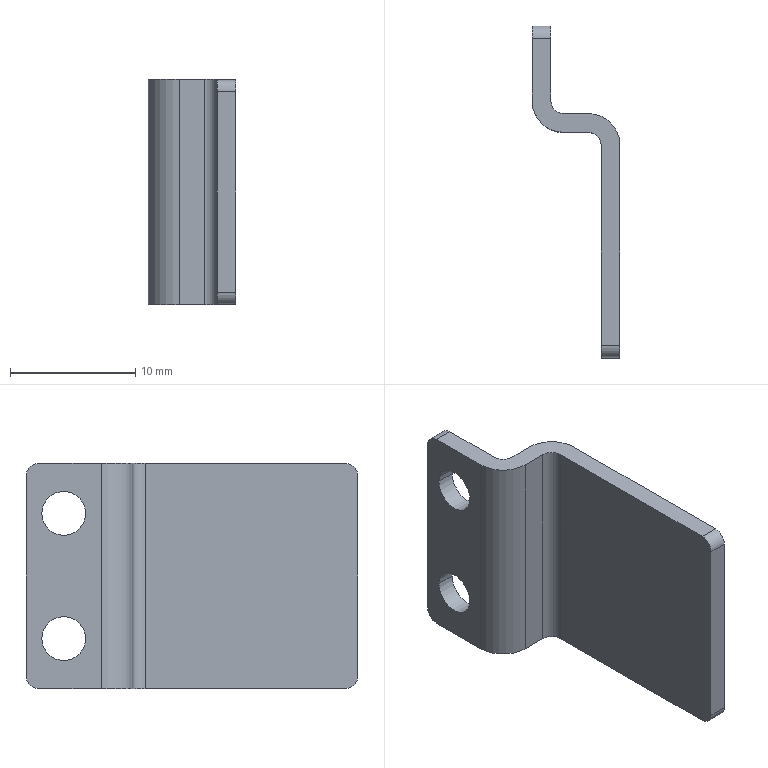Part | SolidWorks | features BaseBody 1 | 1 solid | 22 faces | box 7 x 26.5 x 18 mm | volume 793.289 mm3 | cylinder 12 | plane 10 | commonest cylinder face diameters 2 x6 3.5 x4 5 x2
STEP:
#1=CARTESIAN_POINT('',(-1.5,-4.75,5.));
#2=VERTEX_POINT('',#1);
#3=CARTESIAN_POINT('',(-1.5,-1.25,5.));
#4=VERTEX_POINT('',#3);
#5=CARTESIAN_POINT('',(-1.5,-3.,5.));
#6=DIRECTION('',(1.,0.,0.));
#7=DIRECTION('',(0.,1.,0.));
#8=AXIS2_PLACEMENT_3D('',#5,#6,#7);
#9=CIRCLE('',#8,1.75);
#10=EDGE_CURVE('',#2,#4,#9,.T.);
#11=ORIENTED_EDGE('',*,*,#10,.F.);
#12=CARTESIAN_POINT('',(0.,-4.75,5.));
#13=VERTEX_POINT('',#12);
#14=CARTESIAN_POINT('',(-10.,-4.75,5.));
#15=DIRECTION('',(1.,0.,0.));
#16=VECTOR('',#15,1000.);
#17=LINE('',#14,#16);
#18=EDGE_CURVE('',#2,#13,#17,.T.);
#19=ORIENTED_EDGE('',*,*,#18,.T.);
#20=CARTESIAN_POINT('',(0.,-1.25,5.));
#21=VERTEX_POINT('',#20);
#22=CARTESIAN_POINT('',(0.,-3.,5.));
#23=DIRECTION('',(-1.,0.,0.));
#24=DIRECTION('',(0.,1.,0.));
#25=AXIS2_PLACEMENT_3D('',#22,#23,#24);
#26=CIRCLE('',#25,1.75);
#27=EDGE_CURVE('',#21,#13,#26,.T.);
#28=ORIENTED_EDGE('',*,*,#27,.F.);
#29=CARTESIAN_POINT('',(-10.,-1.25,5.));
#30=DIRECTION('',(1.,0.,0.));
#31=VECTOR('',#30,1000.);
#32=LINE('',#29,#31);
#33=EDGE_CURVE('',#4,#21,#32,.T.);
#34=ORIENTED_EDGE('',*,*,#33,.F.);
#35=EDGE_LOOP('',(#11,#19,#28,#34));
#36=FACE_OUTER_BOUND('',#35,.T.);
#37=CARTESIAN_POINT('',(-10.,-3.,5.));
#38=DIRECTION('',(1.,0.,0.));
#39=DIRECTION('',(0.,1.,0.));
#40=AXIS2_PLACEMENT_3D('',#37,#38,#39);
#41=CYLINDRICAL_SURFACE('',#40,1.75);
#42=ADVANCED_FACE('',(#36),#41,.F.);
#43=CARTESIAN_POINT('',(-1.5,-4.75,-5.));
#44=VERTEX_POINT('',#43);
#45=CARTESIAN_POINT('',(-1.5,-1.25,-5.));
#46=VERTEX_POINT('',#45);
#47=CARTESIAN_POINT('',(-1.5,-3.,-5.));
#48=DIRECTION('',(1.,0.,0.));
#49=DIRECTION('',(0.,1.,0.));
#50=AXIS2_PLACEMENT_3D('',#47,#48,#49);
#51=CIRCLE('',#50,1.75);
#52=EDGE_CURVE('',#44,#46,#51,.T.);
#53=ORIENTED_EDGE('',*,*,#52,.F.);
#54=CARTESIAN_POINT('',(0.,-4.75,-5.));
#55=VERTEX_POINT('',#54);
#56=CARTESIAN_POINT('',(-10.,-4.75,-5.));
#57=DIRECTION('',(1.,0.,0.));
#58=VECTOR('',#57,1000.);
#59=LINE('',#56,#58);
#60=EDGE_CURVE('',#44,#55,#59,.T.);
#61=ORIENTED_EDGE('',*,*,#60,.T.);
#62=CARTESIAN_POINT('',(0.,-1.25,-5.));
#63=VERTEX_POINT('',#62);
#64=CARTESIAN_POINT('',(0.,-3.,-5.));
#65=DIRECTION('',(-1.,0.,0.));
#66=DIRECTION('',(0.,1.,0.));
#67=AXIS2_PLACEMENT_3D('',#64,#65,#66);
#68=CIRCLE('',#67,1.75);
#69=EDGE_CURVE('',#63,#55,#68,.T.);
#70=ORIENTED_EDGE('',*,*,#69,.F.);
#71=CARTESIAN_POINT('',(-10.,-1.25,-5.));
#72=DIRECTION('',(1.,0.,0.));
#73=VECTOR('',#72,1000.);
#74=LINE('',#71,#73);
#75=EDGE_CURVE('',#46,#63,#74,.T.);
#76=ORIENTED_EDGE('',*,*,#75,.F.);
#77=EDGE_LOOP('',(#53,#61,#70,#76));
#78=FACE_OUTER_BOUND('',#77,.T.);
#79=CARTESIAN_POINT('',(-10.,-3.,-5.));
#80=DIRECTION('',(1.,0.,0.));
#81=DIRECTION('',(0.,1.,0.));
#82=AXIS2_PLACEMENT_3D('',#79,#80,#81);
#83=CYLINDRICAL_SURFACE('',#82,1.75);
#84=ADVANCED_FACE('',(#78),#83,.F.);
#85=CARTESIAN_POINT('',(5.5,-25.5,-9.));
#86=VERTEX_POINT('',#85);
#87=CARTESIAN_POINT('',(5.5,-9.5,-9.));
#88=VERTEX_POINT('',#87);
#89=CARTESIAN_POINT('',(5.5,-7.,-9.));
#90=DIRECTION('',(0.,1.,0.));
#91=VECTOR('',#90,1000.);
#92=LINE('',#89,#91);
#93=EDGE_CURVE('',#86,#88,#92,.T.);
#94=ORIENTED_EDGE('',*,*,#93,.T.);
#95=CARTESIAN_POINT('',(5.5,-9.5,9.));
#96=VERTEX_POINT('',#95);
#97=CARTESIAN_POINT('',(5.5,-9.5,9.));
#98=DIRECTION('',(0.,0.,1.));
#99=VECTOR('',#98,1000.);
#100=LINE('',#97,#99);
#101=EDGE_CURVE('',#88,#96,#100,.T.);
#102=ORIENTED_EDGE('',*,*,#101,.T.);
#103=CARTESIAN_POINT('',(5.5,-25.5,9.));
#104=VERTEX_POINT('',#103);
#105=CARTESIAN_POINT('',(5.5,-7.,9.));
#106=DIRECTION('',(0.,-1.,0.));
#107=VECTOR('',#106,1000.);
#108=LINE('',#105,#107);
#109=EDGE_CURVE('',#96,#104,#108,.T.);
#110=ORIENTED_EDGE('',*,*,#109,.T.);
#111=CARTESIAN_POINT('',(5.5,-26.5,8.));
#112=VERTEX_POINT('',#111);
#113=CARTESIAN_POINT('',(5.5,-25.5,8.));
#114=DIRECTION('',(1.,0.,0.));
#115=DIRECTION('',(0.,0.,1.));
#116=AXIS2_PLACEMENT_3D('',#113,#114,#115);
#117=CIRCLE('',#116,1.);
#118=EDGE_CURVE('',#104,#112,#117,.T.);
#119=ORIENTED_EDGE('',*,*,#118,.T.);
#120=CARTESIAN_POINT('',(5.5,-26.5,-8.));
#121=VERTEX_POINT('',#120);
#122=CARTESIAN_POINT('',(5.5,-26.5,9.));
#123=DIRECTION('',(0.,0.,-1.));
#124=VECTOR('',#123,1000.);
#125=LINE('',#122,#124);
#126=EDGE_CURVE('',#112,#121,#125,.T.);
#127=ORIENTED_EDGE('',*,*,#126,.T.);
#128=CARTESIAN_POINT('',(5.5,-25.5,-8.));
#129=DIRECTION('',(1.,0.,0.));
#130=DIRECTION('',(0.,0.,-1.));
#131=AXIS2_PLACEMENT_3D('',#128,#129,#130);
#132=CIRCLE('',#131,1.);
#133=EDGE_CURVE('',#121,#86,#132,.T.);
#134=ORIENTED_EDGE('',*,*,#133,.T.);
#135=EDGE_LOOP('',(#94,#102,#110,#119,#127,#134));
#136=FACE_OUTER_BOUND('',#135,.T.);
#137=CARTESIAN_POINT('',(5.5,-7.,9.));
#138=DIRECTION('',(1.,0.,0.));
#139=DIRECTION('',(0.,1.,0.));
#140=AXIS2_PLACEMENT_3D('',#137,#138,#139);
#141=PLANE('',#140);
#142=ADVANCED_FACE('',(#136),#141,.T.);
#143=CARTESIAN_POINT('',(3.,-7.,9.));
#144=VERTEX_POINT('',#143);
#145=CARTESIAN_POINT('',(3.,-9.5,9.));
#146=DIRECTION('',(0.,0.,-1.));
#147=DIRECTION('',(-1.,0.,0.));
#148=AXIS2_PLACEMENT_3D('',#145,#146,#147);
#149=CIRCLE('',#148,2.5);
#150=EDGE_CURVE('',#144,#96,#149,.T.);
#151=ORIENTED_EDGE('',*,*,#150,.T.);
#152=ORIENTED_EDGE('',*,*,#101,.F.);
#153=CARTESIAN_POINT('',(3.,-7.,-9.));
#154=VERTEX_POINT('',#153);
#155=CARTESIAN_POINT('',(3.,-9.5,-9.));
#156=DIRECTION('',(0.,0.,1.));
#157=DIRECTION('',(-1.,0.,0.));
#158=AXIS2_PLACEMENT_3D('',#155,#156,#157);
#159=CIRCLE('',#158,2.5);
#160=EDGE_CURVE('',#88,#154,#159,.T.);
#161=ORIENTED_EDGE('',*,*,#160,.T.);
#162=CARTESIAN_POINT('',(3.,-7.,9.));
#163=DIRECTION('',(0.,0.,1.));
#164=VECTOR('',#163,1000.);
#165=LINE('',#162,#164);
#166=EDGE_CURVE('',#154,#144,#165,.T.);
#167=ORIENTED_EDGE('',*,*,#166,.T.);
#168=EDGE_LOOP('',(#151,#152,#161,#167));
#169=FACE_OUTER_BOUND('',#168,.T.);
#170=CARTESIAN_POINT('',(3.,-9.5,9.));
#171=DIRECTION('',(0.,0.,-1.));
#172=DIRECTION('',(-1.,0.,0.));
#173=AXIS2_PLACEMENT_3D('',#170,#171,#172);
#174=CYLINDRICAL_SURFACE('',#173,2.5);
#175=ADVANCED_FACE('',(#169),#174,.T.);
#176=CARTESIAN_POINT('',(4.,-25.5,-9.));
#177=VERTEX_POINT('',#176);
#178=CARTESIAN_POINT('',(3.,-25.5,-9.));
#179=DIRECTION('',(1.,0.,0.));
#180=VECTOR('',#179,1000.);
#181=LINE('',#178,#180);
#182=EDGE_CURVE('',#177,#86,#181,.T.);
#183=ORIENTED_EDGE('',*,*,#182,.F.);
#184=CARTESIAN_POINT('',(4.,-9.5,-9.));
#185=VERTEX_POINT('',#184);
#186=CARTESIAN_POINT('',(4.,-9.5,-9.));
#187=DIRECTION('',(0.,-1.,0.));
#188=VECTOR('',#187,1000.);
#189=LINE('',#186,#188);
#190=EDGE_CURVE('',#185,#177,#189,.T.);
#191=ORIENTED_EDGE('',*,*,#190,.F.);
#192=CARTESIAN_POINT('',(3.,-8.5,-9.));
#193=VERTEX_POINT('',#192);
#194=CARTESIAN_POINT('',(3.,-9.5,-9.));
#195=DIRECTION('',(0.,0.,1.));
#196=DIRECTION('',(-1.,0.,0.));
#197=AXIS2_PLACEMENT_3D('',#194,#195,#196);
#198=CIRCLE('',#197,1.);
#199=EDGE_CURVE('',#185,#193,#198,.T.);
#200=ORIENTED_EDGE('',*,*,#199,.T.);
#201=CARTESIAN_POINT('',(1.,-8.5,-9.));
#202=VERTEX_POINT('',#201);
#203=CARTESIAN_POINT('',(4.,-8.5,-9.));
#204=DIRECTION('',(-1.,0.,0.));
#205=VECTOR('',#204,1000.);
#206=LINE('',#203,#205);
#207=EDGE_CURVE('',#193,#202,#206,.T.);
#208=ORIENTED_EDGE('',*,*,#207,.T.);
#209=CARTESIAN_POINT('',(-1.5,-6.,-9.));
#210=VERTEX_POINT('',#209);
#211=CARTESIAN_POINT('',(1.,-6.,-9.));
#212=DIRECTION('',(0.,0.,1.));
#213=DIRECTION('',(-1.,0.,0.));
#214=AXIS2_PLACEMENT_3D('',#211,#212,#213);
#215=CIRCLE('',#214,2.5);
#216=EDGE_CURVE('',#210,#202,#215,.T.);
#217=ORIENTED_EDGE('',*,*,#216,.F.);
#218=CARTESIAN_POINT('',(-1.5,-1.,-9.));
#219=VERTEX_POINT('',#218);
#220=CARTESIAN_POINT('',(-1.5,-8.5,-9.));
#221=DIRECTION('',(0.,1.,0.));
#222=VECTOR('',#221,1000.);
#223=LINE('',#220,#222);
#224=EDGE_CURVE('',#210,#219,#223,.T.);
#225=ORIENTED_EDGE('',*,*,#224,.T.);
#226=CARTESIAN_POINT('',(0.,-1.,-9.));
#227=VERTEX_POINT('',#226);
#228=CARTESIAN_POINT('',(1.,-1.,-9.));
#229=DIRECTION('',(-1.,0.,0.));
#230=VECTOR('',#229,1000.);
#231=LINE('',#228,#230);
#232=EDGE_CURVE('',#227,#219,#231,.T.);
#233=ORIENTED_EDGE('',*,*,#232,.F.);
#234=CARTESIAN_POINT('',(0.,-6.,-9.));
#235=VERTEX_POINT('',#234);
#236=CARTESIAN_POINT('',(0.,0.,-9.));
#237=DIRECTION('',(0.,1.,0.));
#238=VECTOR('',#237,1000.);
#239=LINE('',#236,#238);
#240=EDGE_CURVE('',#235,#227,#239,.T.);
#241=ORIENTED_EDGE('',*,*,#240,.F.);
#242=CARTESIAN_POINT('',(1.,-7.,-9.));
#243=VERTEX_POINT('',#242);
#244=CARTESIAN_POINT('',(1.,-6.,-9.));
#245=DIRECTION('',(0.,0.,1.));
#246=DIRECTION('',(-1.,0.,0.));
#247=AXIS2_PLACEMENT_3D('',#244,#245,#246);
#248=CIRCLE('',#247,1.);
#249=EDGE_CURVE('',#235,#243,#248,.T.);
#250=ORIENTED_EDGE('',*,*,#249,.T.);
#251=CARTESIAN_POINT('',(0.,-7.,-9.));
#252=DIRECTION('',(-1.,0.,0.));
#253=VECTOR('',#252,1000.);
#254=LINE('',#251,#253);
#255=EDGE_CURVE('',#154,#243,#254,.T.);
#256=ORIENTED_EDGE('',*,*,#255,.F.);
#257=ORIENTED_EDGE('',*,*,#160,.F.);
#258=ORIENTED_EDGE('',*,*,#93,.F.);
#259=EDGE_LOOP('',(#183,#191,#200,#208,#217,#225,#233,#241,#250,#256,#257,#258));
#260=FACE_OUTER_BOUND('',#259,.T.);
#261=CARTESIAN_POINT('',(3.,-9.5,-9.));
#262=DIRECTION('',(0.,0.,1.));
#263=DIRECTION('',(1.,0.,0.));
#264=AXIS2_PLACEMENT_3D('',#261,#262,#263);
#265=PLANE('',#264);
#266=ADVANCED_FACE('',(#260),#265,.F.);
#267=CARTESIAN_POINT('',(4.,-26.5,-8.));
#268=VERTEX_POINT('',#267);
#269=CARTESIAN_POINT('',(4.,-25.5,-8.));
#270=DIRECTION('',(1.,0.,0.));
#271=DIRECTION('',(0.,0.,-1.));
#272=AXIS2_PLACEMENT_3D('',#269,#270,#271);
#273=CIRCLE('',#272,1.);
#274=EDGE_CURVE('',#268,#177,#273,.T.);
#275=ORIENTED_EDGE('',*,*,#274,.T.);
#276=ORIENTED_EDGE('',*,*,#182,.T.);
#277=ORIENTED_EDGE('',*,*,#133,.F.);
#278=CARTESIAN_POINT('',(3.,-26.5,-8.));
#279=DIRECTION('',(-1.,0.,0.));
#280=VECTOR('',#279,1000.);
#281=LINE('',#278,#280);
#282=EDGE_CURVE('',#121,#268,#281,.T.);
#283=ORIENTED_EDGE('',*,*,#282,.T.);
#284=EDGE_LOOP('',(#275,#276,#277,#283));
#285=FACE_OUTER_BOUND('',#284,.T.);
#286=CARTESIAN_POINT('',(3.,-25.5,-8.));
#287=DIRECTION('',(1.,0.,0.));
#288=DIRECTION('',(0.,0.,-1.));
#289=AXIS2_PLACEMENT_3D('',#286,#287,#288);
#290=CYLINDRICAL_SURFACE('',#289,1.);
#291=ADVANCED_FACE('',(#285),#290,.T.);
#292=CARTESIAN_POINT('',(4.,-26.5,8.));
#293=VERTEX_POINT('',#292);
#294=CARTESIAN_POINT('',(4.,-26.5,9.));
#295=DIRECTION('',(0.,0.,-1.));
#296=VECTOR('',#295,1000.);
#297=LINE('',#294,#296);
#298=EDGE_CURVE('',#293,#268,#297,.T.);
#299=ORIENTED_EDGE('',*,*,#298,.T.);
#300=ORIENTED_EDGE('',*,*,#282,.F.);
#301=ORIENTED_EDGE('',*,*,#126,.F.);
#302=CARTESIAN_POINT('',(5.5,-26.5,8.));
#303=DIRECTION('',(-1.,0.,0.));
#304=VECTOR('',#303,1000.);
#305=LINE('',#302,#304);
#306=EDGE_CURVE('',#112,#293,#305,.T.);
#307=ORIENTED_EDGE('',*,*,#306,.T.);
#308=EDGE_LOOP('',(#299,#300,#301,#307));
#309=FACE_OUTER_BOUND('',#308,.T.);
#310=CARTESIAN_POINT('',(5.5,-26.5,9.));
#311=DIRECTION('',(0.,-1.,0.));
#312=DIRECTION('',(0.,0.,-1.));
#313=AXIS2_PLACEMENT_3D('',#310,#311,#312);
#314=PLANE('',#313);
#315=ADVANCED_FACE('',(#309),#314,.T.);
#316=CARTESIAN_POINT('',(4.,-25.5,9.));
#317=VERTEX_POINT('',#316);
#318=CARTESIAN_POINT('',(4.,-25.5,8.));
#319=DIRECTION('',(1.,0.,0.));
#320=DIRECTION('',(0.,0.,1.));
#321=AXIS2_PLACEMENT_3D('',#318,#319,#320);
#322=CIRCLE('',#321,1.);
#323=EDGE_CURVE('',#317,#293,#322,.T.);
#324=ORIENTED_EDGE('',*,*,#323,.T.);
#325=ORIENTED_EDGE('',*,*,#306,.F.);
#326=ORIENTED_EDGE('',*,*,#118,.F.);
#327=CARTESIAN_POINT('',(5.5,-25.5,9.));
#328=DIRECTION('',(-1.,0.,0.));
#329=VECTOR('',#328,1000.);
#330=LINE('',#327,#329);
#331=EDGE_CURVE('',#104,#317,#330,.T.);
#332=ORIENTED_EDGE('',*,*,#331,.T.);
#333=EDGE_LOOP('',(#324,#325,#326,#332));
#334=FACE_OUTER_BOUND('',#333,.T.);
#335=CARTESIAN_POINT('',(5.5,-25.5,8.));
#336=DIRECTION('',(-1.,0.,0.));
#337=DIRECTION('',(0.,0.,1.));
#338=AXIS2_PLACEMENT_3D('',#335,#336,#337);
#339=CYLINDRICAL_SURFACE('',#338,1.);
#340=ADVANCED_FACE('',(#334),#339,.T.);
#341=ORIENTED_EDGE('',*,*,#109,.F.);
#342=ORIENTED_EDGE('',*,*,#150,.F.);
#343=CARTESIAN_POINT('',(1.,-7.,9.));
#344=VERTEX_POINT('',#343);
#345=CARTESIAN_POINT('',(0.,-7.,9.));
#346=DIRECTION('',(1.,0.,0.));
#347=VECTOR('',#346,1000.);
#348=LINE('',#345,#347);
#349=EDGE_CURVE('',#344,#144,#348,.T.);
#350=ORIENTED_EDGE('',*,*,#349,.F.);
#351=CARTESIAN_POINT('',(0.,-6.,9.));
#352=VERTEX_POINT('',#351);
#353=CARTESIAN_POINT('',(1.,-6.,9.));
#354=DIRECTION('',(0.,0.,-1.));
#355=DIRECTION('',(-1.,0.,0.));
#356=AXIS2_PLACEMENT_3D('',#353,#354,#355);
#357=CIRCLE('',#356,1.);
#358=EDGE_CURVE('',#344,#352,#357,.T.);
#359=ORIENTED_EDGE('',*,*,#358,.T.);
#360=CARTESIAN_POINT('',(0.,-1.,9.));
#361=VERTEX_POINT('',#360);
#362=CARTESIAN_POINT('',(0.,0.,9.));
#363=DIRECTION('',(0.,-1.,0.));
#364=VECTOR('',#363,1000.);
#365=LINE('',#362,#364);
#366=EDGE_CURVE('',#361,#352,#365,.T.);
#367=ORIENTED_EDGE('',*,*,#366,.F.);
#368=CARTESIAN_POINT('',(-1.5,-1.,9.));
#369=VERTEX_POINT('',#368);
#370=CARTESIAN_POINT('',(3.,-1.,9.));
#371=DIRECTION('',(-1.,0.,0.));
#372=VECTOR('',#371,1000.);
#373=LINE('',#370,#372);
#374=EDGE_CURVE('',#361,#369,#373,.T.);
#375=ORIENTED_EDGE('',*,*,#374,.T.);
#376=CARTESIAN_POINT('',(-1.5,-6.,9.));
#377=VERTEX_POINT('',#376);
#378=CARTESIAN_POINT('',(-1.5,-9.5,9.));
#379=DIRECTION('',(0.,-1.,0.));
#380=VECTOR('',#379,1000.);
#381=LINE('',#378,#380);
#382=EDGE_CURVE('',#369,#377,#381,.T.);
#383=ORIENTED_EDGE('',*,*,#382,.T.);
#384=CARTESIAN_POINT('',(1.,-8.5,9.));
#385=VERTEX_POINT('',#384);
#386=CARTESIAN_POINT('',(1.,-6.,9.));
#387=DIRECTION('',(0.,0.,-1.));
#388=DIRECTION('',(-1.,0.,0.));
#389=AXIS2_PLACEMENT_3D('',#386,#387,#388);
#390=CIRCLE('',#389,2.5);
#391=EDGE_CURVE('',#385,#377,#390,.T.);
#392=ORIENTED_EDGE('',*,*,#391,.F.);
#393=CARTESIAN_POINT('',(3.,-8.5,9.));
#394=VERTEX_POINT('',#393);
#395=CARTESIAN_POINT('',(-1.5,-8.5,9.));
#396=DIRECTION('',(1.,0.,0.));
#397=VECTOR('',#396,1000.);
#398=LINE('',#395,#397);
#399=EDGE_CURVE('',#385,#394,#398,.T.);
#400=ORIENTED_EDGE('',*,*,#399,.T.);
#401=CARTESIAN_POINT('',(4.,-9.5,9.));
#402=VERTEX_POINT('',#401);
#403=CARTESIAN_POINT('',(3.,-9.5,9.));
#404=DIRECTION('',(0.,0.,-1.));
#405=DIRECTION('',(-1.,0.,0.));
#406=AXIS2_PLACEMENT_3D('',#403,#404,#405);
#407=CIRCLE('',#406,1.);
#408=EDGE_CURVE('',#394,#402,#407,.T.);
#409=ORIENTED_EDGE('',*,*,#408,.T.);
#410=CARTESIAN_POINT('',(4.,-8.5,9.));
#411=DIRECTION('',(0.,-1.,0.));
#412=VECTOR('',#411,1000.);
#413=LINE('',#410,#412);
#414=EDGE_CURVE('',#402,#317,#413,.T.);
#415=ORIENTED_EDGE('',*,*,#414,.T.);
#416=ORIENTED_EDGE('',*,*,#331,.F.);
#417=EDGE_LOOP('',(#341,#342,#350,#359,#367,#375,#383,#392,#400,#409,#415,#416));
#418=FACE_OUTER_BOUND('',#417,.T.);
#419=CARTESIAN_POINT('',(3.,-8.5,9.));
#420=DIRECTION('',(0.,0.,1.));
#421=DIRECTION('',(1.,0.,0.));
#422=AXIS2_PLACEMENT_3D('',#419,#420,#421);
#423=PLANE('',#422);
#424=ADVANCED_FACE('',(#418),#423,.T.);
#425=ORIENTED_EDGE('',*,*,#349,.T.);
#426=ORIENTED_EDGE('',*,*,#166,.F.);
#427=ORIENTED_EDGE('',*,*,#255,.T.);
#428=CARTESIAN_POINT('',(1.,-7.,9.));
#429=DIRECTION('',(0.,0.,1.));
#430=VECTOR('',#429,1000.);
#431=LINE('',#428,#430);
#432=EDGE_CURVE('',#243,#344,#431,.T.);
#433=ORIENTED_EDGE('',*,*,#432,.T.);
#434=EDGE_LOOP('',(#425,#426,#427,#433));
#435=FACE_OUTER_BOUND('',#434,.T.);
#436=CARTESIAN_POINT('',(0.,-7.,9.));
#437=DIRECTION('',(0.,1.,0.));
#438=DIRECTION('',(0.,0.,1.));
#439=AXIS2_PLACEMENT_3D('',#436,#437,#438);
#440=PLANE('',#439);
#441=ADVANCED_FACE('',(#435),#440,.T.);
#442=ORIENTED_EDGE('',*,*,#323,.F.);
#443=ORIENTED_EDGE('',*,*,#414,.F.);
#444=CARTESIAN_POINT('',(4.,-9.5,9.));
#445=DIRECTION('',(0.,0.,1.));
#446=VECTOR('',#445,1000.);
#447=LINE('',#444,#446);
#448=EDGE_CURVE('',#185,#402,#447,.T.);
#449=ORIENTED_EDGE('',*,*,#448,.F.);
#450=ORIENTED_EDGE('',*,*,#190,.T.);
#451=ORIENTED_EDGE('',*,*,#274,.F.);
#452=ORIENTED_EDGE('',*,*,#298,.F.);
#453=EDGE_LOOP('',(#442,#443,#449,#450,#451,#452));
#454=FACE_OUTER_BOUND('',#453,.T.);
#455=CARTESIAN_POINT('',(4.,-7.,9.));
#456=DIRECTION('',(1.,0.,0.));
#457=DIRECTION('',(0.,1.,0.));
#458=AXIS2_PLACEMENT_3D('',#455,#456,#457);
#459=PLANE('',#458);
#460=ADVANCED_FACE('',(#454),#459,.F.);
#461=CARTESIAN_POINT('',(0.,-6.,9.));
#462=DIRECTION('',(0.,0.,-1.));
#463=VECTOR('',#462,1000.);
#464=LINE('',#461,#463);
#465=EDGE_CURVE('',#352,#235,#464,.T.);
#466=ORIENTED_EDGE('',*,*,#465,.F.);
#467=ORIENTED_EDGE('',*,*,#358,.F.);
#468=ORIENTED_EDGE('',*,*,#432,.F.);
#469=ORIENTED_EDGE('',*,*,#249,.F.);
#470=EDGE_LOOP('',(#466,#467,#468,#469));
#471=FACE_OUTER_BOUND('',#470,.T.);
#472=CARTESIAN_POINT('',(1.,-6.,9.));
#473=DIRECTION('',(0.,0.,-1.));
#474=DIRECTION('',(-1.,0.,0.));
#475=AXIS2_PLACEMENT_3D('',#472,#473,#474);
#476=CYLINDRICAL_SURFACE('',#475,1.);
#477=ADVANCED_FACE('',(#471),#476,.F.);
#478=ORIENTED_EDGE('',*,*,#448,.T.);
#479=ORIENTED_EDGE('',*,*,#408,.F.);
#480=CARTESIAN_POINT('',(3.,-8.5,9.));
#481=DIRECTION('',(0.,0.,1.));
#482=VECTOR('',#481,1000.);
#483=LINE('',#480,#482);
#484=EDGE_CURVE('',#193,#394,#483,.T.);
#485=ORIENTED_EDGE('',*,*,#484,.F.);
#486=ORIENTED_EDGE('',*,*,#199,.F.);
#487=EDGE_LOOP('',(#478,#479,#485,#486));
#488=FACE_OUTER_BOUND('',#487,.T.);
#489=CARTESIAN_POINT('',(3.,-9.5,9.));
#490=DIRECTION('',(0.,0.,-1.));
#491=DIRECTION('',(-1.,0.,0.));
#492=AXIS2_PLACEMENT_3D('',#489,#490,#491);
#493=CYLINDRICAL_SURFACE('',#492,1.);
#494=ADVANCED_FACE('',(#488),#493,.F.);
#495=ORIENTED_EDGE('',*,*,#484,.T.);
#496=ORIENTED_EDGE('',*,*,#399,.F.);
#497=CARTESIAN_POINT('',(1.,-8.5,9.));
#498=DIRECTION('',(0.,0.,1.));
#499=VECTOR('',#498,1000.);
#500=LINE('',#497,#499);
#501=EDGE_CURVE('',#202,#385,#500,.T.);
#502=ORIENTED_EDGE('',*,*,#501,.F.);
#503=ORIENTED_EDGE('',*,*,#207,.F.);
#504=EDGE_LOOP('',(#495,#496,#502,#503));
#505=FACE_OUTER_BOUND('',#504,.T.);
#506=CARTESIAN_POINT('',(0.,-8.5,9.));
#507=DIRECTION('',(0.,1.,0.));
#508=DIRECTION('',(0.,0.,1.));
#509=AXIS2_PLACEMENT_3D('',#506,#507,#508);
#510=PLANE('',#509);
#511=ADVANCED_FACE('',(#505),#510,.F.);
#512=ORIENTED_EDGE('',*,*,#366,.T.);
#513=ORIENTED_EDGE('',*,*,#465,.T.);
#514=ORIENTED_EDGE('',*,*,#240,.T.);
#515=CARTESIAN_POINT('',(0.,0.,-8.));
#516=VERTEX_POINT('',#515);
#517=CARTESIAN_POINT('',(0.,-1.,-8.));
#518=DIRECTION('',(1.,0.,0.));
#519=DIRECTION('',(0.,1.,0.));
#520=AXIS2_PLACEMENT_3D('',#517,#518,#519);
#521=CIRCLE('',#520,1.);
#522=EDGE_CURVE('',#227,#516,#521,.T.);
#523=ORIENTED_EDGE('',*,*,#522,.T.);
#524=CARTESIAN_POINT('',(0.,0.,8.));
#525=VERTEX_POINT('',#524);
#526=CARTESIAN_POINT('',(0.,0.,9.));
#527=DIRECTION('',(0.,0.,1.));
#528=VECTOR('',#527,1000.);
#529=LINE('',#526,#528);
#530=EDGE_CURVE('',#516,#525,#529,.T.);
#531=ORIENTED_EDGE('',*,*,#530,.T.);
#532=CARTESIAN_POINT('',(0.,-1.,8.));
#533=DIRECTION('',(1.,0.,0.));
#534=DIRECTION('',(0.,1.,0.));
#535=AXIS2_PLACEMENT_3D('',#532,#533,#534);
#536=CIRCLE('',#535,1.);
#537=EDGE_CURVE('',#525,#361,#536,.T.);
#538=ORIENTED_EDGE('',*,*,#537,.T.);
#539=EDGE_LOOP('',(#512,#513,#514,#523,#531,#538));
#540=FACE_OUTER_BOUND('',#539,.T.);
#541=ORIENTED_EDGE('',*,*,#27,.T.);
#542=CARTESIAN_POINT('',(0.,-3.,5.));
#543=DIRECTION('',(-1.,0.,0.));
#544=DIRECTION('',(0.,1.,0.));
#545=AXIS2_PLACEMENT_3D('',#542,#543,#544);
#546=CIRCLE('',#545,1.75);
#547=EDGE_CURVE('',#13,#21,#546,.T.);
#548=ORIENTED_EDGE('',*,*,#547,.T.);
#549=EDGE_LOOP('',(#541,#548));
#550=FACE_BOUND('',#549,.T.);
#551=ORIENTED_EDGE('',*,*,#69,.T.);
#552=CARTESIAN_POINT('',(0.,-3.,-5.));
#553=DIRECTION('',(-1.,0.,0.));
#554=DIRECTION('',(0.,1.,0.));
#555=AXIS2_PLACEMENT_3D('',#552,#553,#554);
#556=CIRCLE('',#555,1.75);
#557=EDGE_CURVE('',#55,#63,#556,.T.);
#558=ORIENTED_EDGE('',*,*,#557,.T.);
#559=EDGE_LOOP('',(#551,#558));
#560=FACE_BOUND('',#559,.T.);
#561=CARTESIAN_POINT('',(0.,0.,9.));
#562=DIRECTION('',(1.,0.,0.));
#563=DIRECTION('',(0.,1.,0.));
#564=AXIS2_PLACEMENT_3D('',#561,#562,#563);
#565=PLANE('',#564);
#566=ADVANCED_FACE('',(#540,#550,#560),#565,.T.);
#567=ORIENTED_EDGE('',*,*,#391,.T.);
#568=CARTESIAN_POINT('',(-1.5,-6.,9.));
#569=DIRECTION('',(0.,0.,-1.));
#570=VECTOR('',#569,1000.);
#571=LINE('',#568,#570);
#572=EDGE_CURVE('',#377,#210,#571,.T.);
#573=ORIENTED_EDGE('',*,*,#572,.T.);
#574=ORIENTED_EDGE('',*,*,#216,.T.);
#575=ORIENTED_EDGE('',*,*,#501,.T.);
#576=EDGE_LOOP('',(#567,#573,#574,#575));
#577=FACE_OUTER_BOUND('',#576,.T.);
#578=CARTESIAN_POINT('',(1.,-6.,9.));
#579=DIRECTION('',(0.,0.,-1.));
#580=DIRECTION('',(-1.,0.,0.));
#581=AXIS2_PLACEMENT_3D('',#578,#579,#580);
#582=CYLINDRICAL_SURFACE('',#581,2.5);
#583=ADVANCED_FACE('',(#577),#582,.T.);
#584=ORIENTED_EDGE('',*,*,#537,.F.);
#585=CARTESIAN_POINT('',(-1.5,0.,8.));
#586=VERTEX_POINT('',#585);
#587=CARTESIAN_POINT('',(-1.5,0.,8.));
#588=DIRECTION('',(-1.,0.,0.));
#589=VECTOR('',#588,1000.);
#590=LINE('',#587,#589);
#591=EDGE_CURVE('',#525,#586,#590,.T.);
#592=ORIENTED_EDGE('',*,*,#591,.T.);
#593=CARTESIAN_POINT('',(-1.5,-1.,8.));
#594=DIRECTION('',(1.,0.,0.));
#595=DIRECTION('',(0.,1.,0.));
#596=AXIS2_PLACEMENT_3D('',#593,#594,#595);
#597=CIRCLE('',#596,1.);
#598=EDGE_CURVE('',#586,#369,#597,.T.);
#599=ORIENTED_EDGE('',*,*,#598,.T.);
#600=ORIENTED_EDGE('',*,*,#374,.F.);
#601=EDGE_LOOP('',(#584,#592,#599,#600));
#602=FACE_OUTER_BOUND('',#601,.T.);
#603=CARTESIAN_POINT('',(-1.5,-1.,8.));
#604=DIRECTION('',(1.,0.,0.));
#605=DIRECTION('',(0.,1.,0.));
#606=AXIS2_PLACEMENT_3D('',#603,#604,#605);
#607=CYLINDRICAL_SURFACE('',#606,1.);
#608=ADVANCED_FACE('',(#602),#607,.T.);
#609=CARTESIAN_POINT('',(-1.5,0.,-8.));
#610=VERTEX_POINT('',#609);
#611=CARTESIAN_POINT('',(-1.5,0.,9.));
#612=DIRECTION('',(0.,0.,1.));
#613=VECTOR('',#612,1000.);
#614=LINE('',#611,#613);
#615=EDGE_CURVE('',#610,#586,#614,.T.);
#616=ORIENTED_EDGE('',*,*,#615,.T.);
#617=ORIENTED_EDGE('',*,*,#591,.F.);
#618=ORIENTED_EDGE('',*,*,#530,.F.);
#619=CARTESIAN_POINT('',(-1.5,0.,-8.));
#620=DIRECTION('',(-1.,0.,0.));
#621=VECTOR('',#620,1000.);
#622=LINE('',#619,#621);
#623=EDGE_CURVE('',#516,#610,#622,.T.);
#624=ORIENTED_EDGE('',*,*,#623,.T.);
#625=EDGE_LOOP('',(#616,#617,#618,#624));
#626=FACE_OUTER_BOUND('',#625,.T.);
#627=CARTESIAN_POINT('',(-1.5,0.,9.));
#628=DIRECTION('',(0.,1.,0.));
#629=DIRECTION('',(-1.,0.,0.));
#630=AXIS2_PLACEMENT_3D('',#627,#628,#629);
#631=PLANE('',#630);
#632=ADVANCED_FACE('',(#626),#631,.T.);
#633=ORIENTED_EDGE('',*,*,#522,.F.);
#634=ORIENTED_EDGE('',*,*,#232,.T.);
#635=CARTESIAN_POINT('',(-1.5,-1.,-8.));
#636=DIRECTION('',(1.,0.,0.));
#637=DIRECTION('',(0.,1.,0.));
#638=AXIS2_PLACEMENT_3D('',#635,#636,#637);
#639=CIRCLE('',#638,1.);
#640=EDGE_CURVE('',#219,#610,#639,.T.);
#641=ORIENTED_EDGE('',*,*,#640,.T.);
#642=ORIENTED_EDGE('',*,*,#623,.F.);
#643=EDGE_LOOP('',(#633,#634,#641,#642));
#644=FACE_OUTER_BOUND('',#643,.T.);
#645=CARTESIAN_POINT('',(1.,-1.,-8.));
#646=DIRECTION('',(1.,0.,0.));
#647=DIRECTION('',(0.,1.,0.));
#648=AXIS2_PLACEMENT_3D('',#645,#646,#647);
#649=CYLINDRICAL_SURFACE('',#648,1.);
#650=ADVANCED_FACE('',(#644),#649,.T.);
#651=ORIENTED_EDGE('',*,*,#18,.F.);
#652=CARTESIAN_POINT('',(-1.5,-3.,5.));
#653=DIRECTION('',(1.,0.,0.));
#654=DIRECTION('',(0.,1.,0.));
#655=AXIS2_PLACEMENT_3D('',#652,#653,#654);
#656=CIRCLE('',#655,1.75);
#657=EDGE_CURVE('',#4,#2,#656,.T.);
#658=ORIENTED_EDGE('',*,*,#657,.F.);
#659=ORIENTED_EDGE('',*,*,#33,.T.);
#660=ORIENTED_EDGE('',*,*,#547,.F.);
#661=EDGE_LOOP('',(#651,#658,#659,#660));
#662=FACE_OUTER_BOUND('',#661,.T.);
#663=CARTESIAN_POINT('',(-10.,-3.,5.));
#664=DIRECTION('',(1.,0.,0.));
#665=DIRECTION('',(0.,1.,0.));
#666=AXIS2_PLACEMENT_3D('',#663,#664,#665);
#667=CYLINDRICAL_SURFACE('',#666,1.75);
#668=ADVANCED_FACE('',(#662),#667,.F.);
#669=ORIENTED_EDGE('',*,*,#60,.F.);
#670=CARTESIAN_POINT('',(-1.5,-3.,-5.));
#671=DIRECTION('',(1.,0.,0.));
#672=DIRECTION('',(0.,1.,0.));
#673=AXIS2_PLACEMENT_3D('',#670,#671,#672);
#674=CIRCLE('',#673,1.75);
#675=EDGE_CURVE('',#46,#44,#674,.T.);
#676=ORIENTED_EDGE('',*,*,#675,.F.);
#677=ORIENTED_EDGE('',*,*,#75,.T.);
#678=ORIENTED_EDGE('',*,*,#557,.F.);
#679=EDGE_LOOP('',(#669,#676,#677,#678));
#680=FACE_OUTER_BOUND('',#679,.T.);
#681=CARTESIAN_POINT('',(-10.,-3.,-5.));
#682=DIRECTION('',(1.,0.,0.));
#683=DIRECTION('',(0.,1.,0.));
#684=AXIS2_PLACEMENT_3D('',#681,#682,#683);
#685=CYLINDRICAL_SURFACE('',#684,1.75);
#686=ADVANCED_FACE('',(#680),#685,.F.);
#687=ORIENTED_EDGE('',*,*,#640,.F.);
#688=ORIENTED_EDGE('',*,*,#224,.F.);
#689=ORIENTED_EDGE('',*,*,#572,.F.);
#690=ORIENTED_EDGE('',*,*,#382,.F.);
#691=ORIENTED_EDGE('',*,*,#598,.F.);
#692=ORIENTED_EDGE('',*,*,#615,.F.);
#693=EDGE_LOOP('',(#687,#688,#689,#690,#691,#692));
#694=FACE_OUTER_BOUND('',#693,.T.);
#695=ORIENTED_EDGE('',*,*,#657,.T.);
#696=ORIENTED_EDGE('',*,*,#10,.T.);
#697=EDGE_LOOP('',(#695,#696));
#698=FACE_BOUND('',#697,.T.);
#699=ORIENTED_EDGE('',*,*,#675,.T.);
#700=ORIENTED_EDGE('',*,*,#52,.T.);
#701=EDGE_LOOP('',(#699,#700));
#702=FACE_BOUND('',#701,.T.);
#703=CARTESIAN_POINT('',(-1.5,0.,9.));
#704=DIRECTION('',(1.,0.,0.));
#705=DIRECTION('',(0.,1.,0.));
#706=AXIS2_PLACEMENT_3D('',#703,#704,#705);
#707=PLANE('',#706);
#708=ADVANCED_FACE('',(#694,#698,#702),#707,.F.);
#709=CLOSED_SHELL('',(#42,#84,#142,#175,#266,#291,#315,#340,#424,#441,#460,#477,#494,#511,#566,#583,#608,#632,#650,#668,#686,#708));
#710=MANIFOLD_SOLID_BREP('',#709);
#711=CARTESIAN_POINT('',(0.,0.,0.));
#712=DIRECTION('',(0.,0.,1.));
#713=DIRECTION('',(1.,0.,0.));
#714=AXIS2_PLACEMENT_3D('',#711,#712,#713);
#715=(LENGTH_UNIT()NAMED_UNIT(*)SI_UNIT(.MILLI.,.METRE.));
#716=UNCERTAINTY_MEASURE_WITH_UNIT(LENGTH_MEASURE(0.00001),#715,'','');
#717=(NAMED_UNIT(*)PLANE_ANGLE_UNIT()SI_UNIT($,.RADIAN.));
#718=(NAMED_UNIT(*)SI_UNIT($,.STERADIAN.)SOLID_ANGLE_UNIT());
#719=(GEOMETRIC_REPRESENTATION_CONTEXT(3)GLOBAL_UNCERTAINTY_ASSIGNED_CONTEXT((#716))GLOBAL_UNIT_ASSIGNED_CONTEXT((#715,#717,#718))REPRESENTATION_CONTEXT('',''));
#720=ADVANCED_BREP_SHAPE_REPRESENTATION('',(#710,#714),#719);